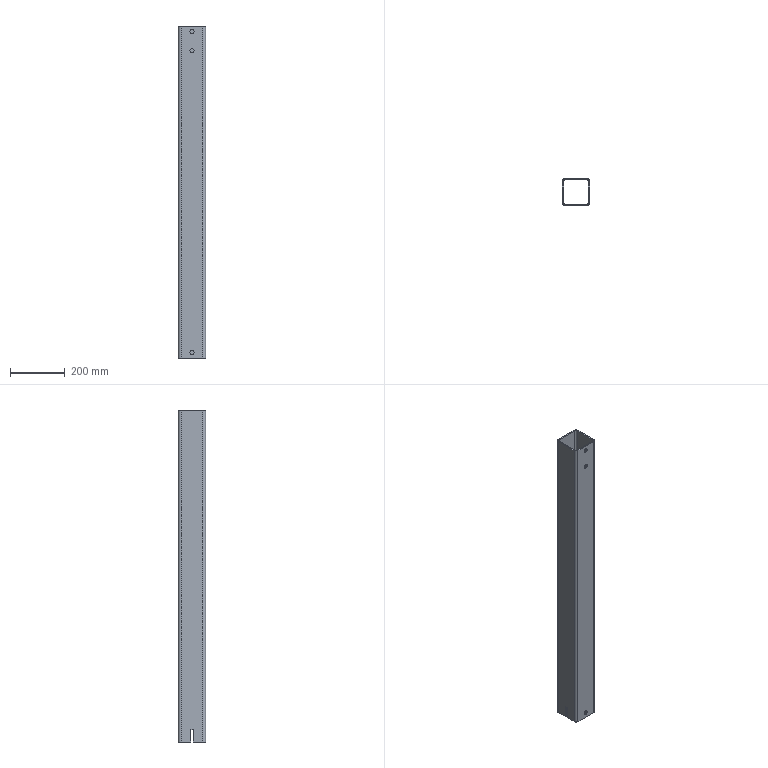Part | SolidWorks | features ICE 4, Attribute 1, Extrusion 1 | 1 solid | 39 faces | box 100 x 100 x 1211 mm | volume 1999990 mm3 | cylinder 22 | plane 17 | commonest cylinder face diameters 15 x14 11 x4 20 x4
STEP:
#1=CARTESIAN_POINT('',(-15.,45.5,1163.5));
#2=VERTEX_POINT('',#1);
#3=CARTESIAN_POINT('',(-15.,45.5,1178.5));
#4=VERTEX_POINT('',#3);
#5=CARTESIAN_POINT('',(-15.,45.5,1171.));
#6=DIRECTION('',(0.,1.,0.));
#7=DIRECTION('',(0.,0.,-1.));
#8=AXIS2_PLACEMENT_3D('',#5,#6,#7);
#9=CIRCLE('',#8,7.5);
#10=EDGE_CURVE('',#2,#4,#9,.T.);
#11=ORIENTED_EDGE('',*,*,#10,.F.);
#12=CARTESIAN_POINT('',(-15.,50.,1163.5));
#13=VERTEX_POINT('',#12);
#14=CARTESIAN_POINT('',(-15.,-50.001,1163.5));
#15=DIRECTION('',(0.,1.,0.));
#16=VECTOR('',#15,1000.);
#17=LINE('',#14,#16);
#18=EDGE_CURVE('',#2,#13,#17,.T.);
#19=ORIENTED_EDGE('',*,*,#18,.T.);
#20=CARTESIAN_POINT('',(-15.,50.,1178.5));
#21=VERTEX_POINT('',#20);
#22=CARTESIAN_POINT('',(-15.,50.,1171.));
#23=DIRECTION('',(0.,1.,0.));
#24=DIRECTION('',(0.,0.,1.));
#25=AXIS2_PLACEMENT_3D('',#22,#23,#24);
#26=CIRCLE('',#25,7.5);
#27=EDGE_CURVE('',#13,#21,#26,.T.);
#28=ORIENTED_EDGE('',*,*,#27,.T.);
#29=CARTESIAN_POINT('',(-15.,-50.001,1178.5));
#30=DIRECTION('',(0.,1.,0.));
#31=VECTOR('',#30,1000.);
#32=LINE('',#29,#31);
#33=EDGE_CURVE('',#4,#21,#32,.T.);
#34=ORIENTED_EDGE('',*,*,#33,.F.);
#35=EDGE_LOOP('',(#11,#19,#28,#34));
#36=FACE_OUTER_BOUND('',#35,.T.);
#37=CARTESIAN_POINT('',(-15.,-50.001,1171.));
#38=DIRECTION('',(0.,1.,0.));
#39=DIRECTION('',(0.,0.,1.));
#40=AXIS2_PLACEMENT_3D('',#37,#38,#39);
#41=CYLINDRICAL_SURFACE('',#40,7.5);
#42=ADVANCED_FACE('',(#36),#41,.F.);
#43=CARTESIAN_POINT('',(-15.,45.5,1113.5));
#44=VERTEX_POINT('',#43);
#45=CARTESIAN_POINT('',(-15.,45.5,1128.5));
#46=VERTEX_POINT('',#45);
#47=CARTESIAN_POINT('',(-15.,45.5,1121.));
#48=DIRECTION('',(0.,1.,0.));
#49=DIRECTION('',(0.,0.,-1.));
#50=AXIS2_PLACEMENT_3D('',#47,#48,#49);
#51=CIRCLE('',#50,7.5);
#52=EDGE_CURVE('',#44,#46,#51,.T.);
#53=ORIENTED_EDGE('',*,*,#52,.F.);
#54=CARTESIAN_POINT('',(-15.,50.,1113.5));
#55=VERTEX_POINT('',#54);
#56=CARTESIAN_POINT('',(-15.,-50.001,1113.5));
#57=DIRECTION('',(0.,1.,0.));
#58=VECTOR('',#57,1000.);
#59=LINE('',#56,#58);
#60=EDGE_CURVE('',#44,#55,#59,.T.);
#61=ORIENTED_EDGE('',*,*,#60,.T.);
#62=CARTESIAN_POINT('',(-15.,50.,1128.5));
#63=VERTEX_POINT('',#62);
#64=CARTESIAN_POINT('',(-15.,50.,1121.));
#65=DIRECTION('',(0.,1.,0.));
#66=DIRECTION('',(0.,0.,1.));
#67=AXIS2_PLACEMENT_3D('',#64,#65,#66);
#68=CIRCLE('',#67,7.5);
#69=EDGE_CURVE('',#55,#63,#68,.T.);
#70=ORIENTED_EDGE('',*,*,#69,.T.);
#71=CARTESIAN_POINT('',(-15.,-50.001,1128.5));
#72=DIRECTION('',(0.,1.,0.));
#73=VECTOR('',#72,1000.);
#74=LINE('',#71,#73);
#75=EDGE_CURVE('',#46,#63,#74,.T.);
#76=ORIENTED_EDGE('',*,*,#75,.F.);
#77=EDGE_LOOP('',(#53,#61,#70,#76));
#78=FACE_OUTER_BOUND('',#77,.T.);
#79=CARTESIAN_POINT('',(-15.,-50.001,1121.));
#80=DIRECTION('',(0.,1.,0.));
#81=DIRECTION('',(0.,0.,1.));
#82=AXIS2_PLACEMENT_3D('',#79,#80,#81);
#83=CYLINDRICAL_SURFACE('',#82,7.5);
#84=ADVANCED_FACE('',(#78),#83,.F.);
#85=CARTESIAN_POINT('',(0.,-45.5,1198.5));
#86=VERTEX_POINT('',#85);
#87=CARTESIAN_POINT('',(0.,-45.5,1183.5));
#88=VERTEX_POINT('',#87);
#89=CARTESIAN_POINT('',(0.,-45.5,1191.));
#90=DIRECTION('',(0.,-1.,0.));
#91=DIRECTION('',(0.,0.,1.));
#92=AXIS2_PLACEMENT_3D('',#89,#90,#91);
#93=CIRCLE('',#92,7.5);
#94=EDGE_CURVE('',#86,#88,#93,.T.);
#95=ORIENTED_EDGE('',*,*,#94,.F.);
#96=CARTESIAN_POINT('',(0.,-50.,1198.5));
#97=VERTEX_POINT('',#96);
#98=CARTESIAN_POINT('',(0.,50.001,1198.5));
#99=DIRECTION('',(0.,-1.,0.));
#100=VECTOR('',#99,1000.);
#101=LINE('',#98,#100);
#102=EDGE_CURVE('',#86,#97,#101,.T.);
#103=ORIENTED_EDGE('',*,*,#102,.T.);
#104=CARTESIAN_POINT('',(0.,-50.,1183.5));
#105=VERTEX_POINT('',#104);
#106=CARTESIAN_POINT('',(0.,-50.,1191.));
#107=DIRECTION('',(0.,-1.,0.));
#108=DIRECTION('',(0.,0.,-1.));
#109=AXIS2_PLACEMENT_3D('',#106,#107,#108);
#110=CIRCLE('',#109,7.5);
#111=EDGE_CURVE('',#97,#105,#110,.T.);
#112=ORIENTED_EDGE('',*,*,#111,.T.);
#113=CARTESIAN_POINT('',(0.,50.001,1183.5));
#114=DIRECTION('',(0.,-1.,0.));
#115=VECTOR('',#114,1000.);
#116=LINE('',#113,#115);
#117=EDGE_CURVE('',#88,#105,#116,.T.);
#118=ORIENTED_EDGE('',*,*,#117,.F.);
#119=EDGE_LOOP('',(#95,#103,#112,#118));
#120=FACE_OUTER_BOUND('',#119,.T.);
#121=CARTESIAN_POINT('',(0.,50.001,1191.));
#122=DIRECTION('',(0.,-1.,0.));
#123=DIRECTION('',(0.,0.,-1.));
#124=AXIS2_PLACEMENT_3D('',#121,#122,#123);
#125=CYLINDRICAL_SURFACE('',#124,7.5);
#126=ADVANCED_FACE('',(#120),#125,.F.);
#127=CARTESIAN_POINT('',(0.,-45.5,1128.5));
#128=VERTEX_POINT('',#127);
#129=CARTESIAN_POINT('',(0.,-45.5,1113.5));
#130=VERTEX_POINT('',#129);
#131=CARTESIAN_POINT('',(0.,-45.5,1121.));
#132=DIRECTION('',(0.,-1.,0.));
#133=DIRECTION('',(0.,0.,1.));
#134=AXIS2_PLACEMENT_3D('',#131,#132,#133);
#135=CIRCLE('',#134,7.5);
#136=EDGE_CURVE('',#128,#130,#135,.T.);
#137=ORIENTED_EDGE('',*,*,#136,.F.);
#138=CARTESIAN_POINT('',(0.,-50.,1128.5));
#139=VERTEX_POINT('',#138);
#140=CARTESIAN_POINT('',(0.,50.001,1128.5));
#141=DIRECTION('',(0.,-1.,0.));
#142=VECTOR('',#141,1000.);
#143=LINE('',#140,#142);
#144=EDGE_CURVE('',#128,#139,#143,.T.);
#145=ORIENTED_EDGE('',*,*,#144,.T.);
#146=CARTESIAN_POINT('',(0.,-50.,1113.5));
#147=VERTEX_POINT('',#146);
#148=CARTESIAN_POINT('',(0.,-50.,1121.));
#149=DIRECTION('',(0.,-1.,0.));
#150=DIRECTION('',(0.,0.,-1.));
#151=AXIS2_PLACEMENT_3D('',#148,#149,#150);
#152=CIRCLE('',#151,7.5);
#153=EDGE_CURVE('',#139,#147,#152,.T.);
#154=ORIENTED_EDGE('',*,*,#153,.T.);
#155=CARTESIAN_POINT('',(0.,50.001,1113.5));
#156=DIRECTION('',(0.,-1.,0.));
#157=VECTOR('',#156,1000.);
#158=LINE('',#155,#157);
#159=EDGE_CURVE('',#130,#147,#158,.T.);
#160=ORIENTED_EDGE('',*,*,#159,.F.);
#161=EDGE_LOOP('',(#137,#145,#154,#160));
#162=FACE_OUTER_BOUND('',#161,.T.);
#163=CARTESIAN_POINT('',(0.,50.001,1121.));
#164=DIRECTION('',(0.,-1.,0.));
#165=DIRECTION('',(0.,0.,-1.));
#166=AXIS2_PLACEMENT_3D('',#163,#164,#165);
#167=CYLINDRICAL_SURFACE('',#166,7.5);
#168=ADVANCED_FACE('',(#162),#167,.F.);
#169=CARTESIAN_POINT('',(0.,-45.5,27.5));
#170=VERTEX_POINT('',#169);
#171=CARTESIAN_POINT('',(0.,-45.5,12.5));
#172=VERTEX_POINT('',#171);
#173=CARTESIAN_POINT('',(0.,-45.5,20.));
#174=DIRECTION('',(0.,-1.,0.));
#175=DIRECTION('',(0.,0.,1.));
#176=AXIS2_PLACEMENT_3D('',#173,#174,#175);
#177=CIRCLE('',#176,7.5);
#178=EDGE_CURVE('',#170,#172,#177,.T.);
#179=ORIENTED_EDGE('',*,*,#178,.F.);
#180=CARTESIAN_POINT('',(0.,-50.,27.5));
#181=VERTEX_POINT('',#180);
#182=CARTESIAN_POINT('',(0.,50.001,27.5));
#183=DIRECTION('',(0.,-1.,0.));
#184=VECTOR('',#183,1000.);
#185=LINE('',#182,#184);
#186=EDGE_CURVE('',#170,#181,#185,.T.);
#187=ORIENTED_EDGE('',*,*,#186,.T.);
#188=CARTESIAN_POINT('',(0.,-50.,12.5));
#189=VERTEX_POINT('',#188);
#190=CARTESIAN_POINT('',(0.,-50.,20.));
#191=DIRECTION('',(0.,-1.,0.));
#192=DIRECTION('',(0.,0.,-1.));
#193=AXIS2_PLACEMENT_3D('',#190,#191,#192);
#194=CIRCLE('',#193,7.5);
#195=EDGE_CURVE('',#181,#189,#194,.T.);
#196=ORIENTED_EDGE('',*,*,#195,.T.);
#197=CARTESIAN_POINT('',(0.,50.001,12.5));
#198=DIRECTION('',(0.,-1.,0.));
#199=VECTOR('',#198,1000.);
#200=LINE('',#197,#199);
#201=EDGE_CURVE('',#172,#189,#200,.T.);
#202=ORIENTED_EDGE('',*,*,#201,.F.);
#203=EDGE_LOOP('',(#179,#187,#196,#202));
#204=FACE_OUTER_BOUND('',#203,.T.);
#205=CARTESIAN_POINT('',(0.,50.001,20.));
#206=DIRECTION('',(0.,-1.,0.));
#207=DIRECTION('',(0.,0.,-1.));
#208=AXIS2_PLACEMENT_3D('',#205,#206,#207);
#209=CYLINDRICAL_SURFACE('',#208,7.5);
#210=ADVANCED_FACE('',(#204),#209,.F.);
#211=CARTESIAN_POINT('',(45.5,-15.,1178.5));
#212=VERTEX_POINT('',#211);
#213=CARTESIAN_POINT('',(45.5,-15.,1163.5));
#214=VERTEX_POINT('',#213);
#215=CARTESIAN_POINT('',(45.5,-15.,1171.));
#216=DIRECTION('',(1.,0.,0.));
#217=DIRECTION('',(0.,0.,1.));
#218=AXIS2_PLACEMENT_3D('',#215,#216,#217);
#219=CIRCLE('',#218,7.5);
#220=EDGE_CURVE('',#212,#214,#219,.T.);
#221=ORIENTED_EDGE('',*,*,#220,.F.);
#222=CARTESIAN_POINT('',(50.,-15.,1178.5));
#223=VERTEX_POINT('',#222);
#224=CARTESIAN_POINT('',(-50.001,-15.,1178.5));
#225=DIRECTION('',(1.,0.,0.));
#226=VECTOR('',#225,1000.);
#227=LINE('',#224,#226);
#228=EDGE_CURVE('',#212,#223,#227,.T.);
#229=ORIENTED_EDGE('',*,*,#228,.T.);
#230=CARTESIAN_POINT('',(50.,-15.,1163.5));
#231=VERTEX_POINT('',#230);
#232=CARTESIAN_POINT('',(50.,-15.,1171.));
#233=DIRECTION('',(1.,0.,0.));
#234=DIRECTION('',(0.,0.,-1.));
#235=AXIS2_PLACEMENT_3D('',#232,#233,#234);
#236=CIRCLE('',#235,7.5);
#237=EDGE_CURVE('',#223,#231,#236,.T.);
#238=ORIENTED_EDGE('',*,*,#237,.T.);
#239=CARTESIAN_POINT('',(-50.001,-15.,1163.5));
#240=DIRECTION('',(1.,0.,0.));
#241=VECTOR('',#240,1000.);
#242=LINE('',#239,#241);
#243=EDGE_CURVE('',#214,#231,#242,.T.);
#244=ORIENTED_EDGE('',*,*,#243,.F.);
#245=EDGE_LOOP('',(#221,#229,#238,#244));
#246=FACE_OUTER_BOUND('',#245,.T.);
#247=CARTESIAN_POINT('',(-50.001,-15.,1171.));
#248=DIRECTION('',(1.,0.,0.));
#249=DIRECTION('',(0.,0.,-1.));
#250=AXIS2_PLACEMENT_3D('',#247,#248,#249);
#251=CYLINDRICAL_SURFACE('',#250,7.5);
#252=ADVANCED_FACE('',(#246),#251,.F.);
#253=CARTESIAN_POINT('',(45.5,-15.,1128.5));
#254=VERTEX_POINT('',#253);
#255=CARTESIAN_POINT('',(45.5,-15.,1113.5));
#256=VERTEX_POINT('',#255);
#257=CARTESIAN_POINT('',(45.5,-15.,1121.));
#258=DIRECTION('',(1.,0.,0.));
#259=DIRECTION('',(0.,0.,1.));
#260=AXIS2_PLACEMENT_3D('',#257,#258,#259);
#261=CIRCLE('',#260,7.5);
#262=EDGE_CURVE('',#254,#256,#261,.T.);
#263=ORIENTED_EDGE('',*,*,#262,.F.);
#264=CARTESIAN_POINT('',(50.,-15.,1128.5));
#265=VERTEX_POINT('',#264);
#266=CARTESIAN_POINT('',(-50.001,-15.,1128.5));
#267=DIRECTION('',(1.,0.,0.));
#268=VECTOR('',#267,1000.);
#269=LINE('',#266,#268);
#270=EDGE_CURVE('',#254,#265,#269,.T.);
#271=ORIENTED_EDGE('',*,*,#270,.T.);
#272=CARTESIAN_POINT('',(50.,-15.,1113.5));
#273=VERTEX_POINT('',#272);
#274=CARTESIAN_POINT('',(50.,-15.,1121.));
#275=DIRECTION('',(1.,0.,0.));
#276=DIRECTION('',(0.,0.,-1.));
#277=AXIS2_PLACEMENT_3D('',#274,#275,#276);
#278=CIRCLE('',#277,7.5);
#279=EDGE_CURVE('',#265,#273,#278,.T.);
#280=ORIENTED_EDGE('',*,*,#279,.T.);
#281=CARTESIAN_POINT('',(-50.001,-15.,1113.5));
#282=DIRECTION('',(1.,0.,0.));
#283=VECTOR('',#282,1000.);
#284=LINE('',#281,#283);
#285=EDGE_CURVE('',#256,#273,#284,.T.);
#286=ORIENTED_EDGE('',*,*,#285,.F.);
#287=EDGE_LOOP('',(#263,#271,#280,#286));
#288=FACE_OUTER_BOUND('',#287,.T.);
#289=CARTESIAN_POINT('',(-50.001,-15.,1121.));
#290=DIRECTION('',(1.,0.,0.));
#291=DIRECTION('',(0.,0.,-1.));
#292=AXIS2_PLACEMENT_3D('',#289,#290,#291);
#293=CYLINDRICAL_SURFACE('',#292,7.5);
#294=ADVANCED_FACE('',(#288),#293,.F.);
#295=CARTESIAN_POINT('',(-50.,-4.5,0.));
#296=VERTEX_POINT('',#295);
#297=CARTESIAN_POINT('',(-50.,-40.,0.));
#298=VERTEX_POINT('',#297);
#299=CARTESIAN_POINT('',(-50.,-40.,0.));
#300=DIRECTION('',(0.,-1.,0.));
#301=VECTOR('',#300,1000.);
#302=LINE('',#299,#301);
#303=EDGE_CURVE('',#296,#298,#302,.T.);
#304=ORIENTED_EDGE('',*,*,#303,.F.);
#305=CARTESIAN_POINT('',(-45.5,-4.5,0.));
#306=VERTEX_POINT('',#305);
#307=CARTESIAN_POINT('',(-50.,-4.5,0.));
#308=DIRECTION('',(1.,0.,0.));
#309=VECTOR('',#308,1000.);
#310=LINE('',#307,#309);
#311=EDGE_CURVE('',#296,#306,#310,.T.);
#312=ORIENTED_EDGE('',*,*,#311,.T.);
#313=CARTESIAN_POINT('',(-45.5,-40.,0.));
#314=VERTEX_POINT('',#313);
#315=CARTESIAN_POINT('',(-45.5,-40.,0.));
#316=DIRECTION('',(0.,-1.,0.));
#317=VECTOR('',#316,1000.);
#318=LINE('',#315,#317);
#319=EDGE_CURVE('',#306,#314,#318,.T.);
#320=ORIENTED_EDGE('',*,*,#319,.T.);
#321=CARTESIAN_POINT('',(-40.,-45.5,0.));
#322=VERTEX_POINT('',#321);
#323=CARTESIAN_POINT('',(-40.,-40.,0.));
#324=DIRECTION('',(0.,0.,1.));
#325=DIRECTION('',(1.,0.,0.));
#326=AXIS2_PLACEMENT_3D('',#323,#324,#325);
#327=CIRCLE('',#326,5.5);
#328=EDGE_CURVE('',#314,#322,#327,.T.);
#329=ORIENTED_EDGE('',*,*,#328,.T.);
#330=CARTESIAN_POINT('',(40.,-45.5,0.));
#331=VERTEX_POINT('',#330);
#332=CARTESIAN_POINT('',(-40.,-45.5,0.));
#333=DIRECTION('',(1.,0.,0.));
#334=VECTOR('',#333,1000.);
#335=LINE('',#332,#334);
#336=EDGE_CURVE('',#322,#331,#335,.T.);
#337=ORIENTED_EDGE('',*,*,#336,.T.);
#338=CARTESIAN_POINT('',(45.5,-40.,0.));
#339=VERTEX_POINT('',#338);
#340=CARTESIAN_POINT('',(40.,-40.,0.));
#341=DIRECTION('',(0.,0.,1.));
#342=DIRECTION('',(1.,0.,0.));
#343=AXIS2_PLACEMENT_3D('',#340,#341,#342);
#344=CIRCLE('',#343,5.5);
#345=EDGE_CURVE('',#331,#339,#344,.T.);
#346=ORIENTED_EDGE('',*,*,#345,.T.);
#347=CARTESIAN_POINT('',(45.5,-4.5,0.));
#348=VERTEX_POINT('',#347);
#349=CARTESIAN_POINT('',(45.5,40.,0.));
#350=DIRECTION('',(0.,1.,0.));
#351=VECTOR('',#350,1000.);
#352=LINE('',#349,#351);
#353=EDGE_CURVE('',#339,#348,#352,.T.);
#354=ORIENTED_EDGE('',*,*,#353,.T.);
#355=CARTESIAN_POINT('',(50.,-4.5,0.));
#356=VERTEX_POINT('',#355);
#357=CARTESIAN_POINT('',(-50.,-4.5,0.));
#358=DIRECTION('',(1.,0.,0.));
#359=VECTOR('',#358,1000.);
#360=LINE('',#357,#359);
#361=EDGE_CURVE('',#348,#356,#360,.T.);
#362=ORIENTED_EDGE('',*,*,#361,.T.);
#363=CARTESIAN_POINT('',(50.,-40.,0.));
#364=VERTEX_POINT('',#363);
#365=CARTESIAN_POINT('',(50.,40.,0.));
#366=DIRECTION('',(0.,1.,0.));
#367=VECTOR('',#366,1000.);
#368=LINE('',#365,#367);
#369=EDGE_CURVE('',#364,#356,#368,.T.);
#370=ORIENTED_EDGE('',*,*,#369,.F.);
#371=CARTESIAN_POINT('',(40.,-50.,0.));
#372=VERTEX_POINT('',#371);
#373=CARTESIAN_POINT('',(40.,-40.,0.));
#374=DIRECTION('',(0.,0.,1.));
#375=DIRECTION('',(1.,0.,0.));
#376=AXIS2_PLACEMENT_3D('',#373,#374,#375);
#377=CIRCLE('',#376,10.);
#378=EDGE_CURVE('',#372,#364,#377,.T.);
#379=ORIENTED_EDGE('',*,*,#378,.F.);
#380=CARTESIAN_POINT('',(-40.,-50.,0.));
#381=VERTEX_POINT('',#380);
#382=CARTESIAN_POINT('',(-40.,-50.,0.));
#383=DIRECTION('',(1.,0.,0.));
#384=VECTOR('',#383,1000.);
#385=LINE('',#382,#384);
#386=EDGE_CURVE('',#381,#372,#385,.T.);
#387=ORIENTED_EDGE('',*,*,#386,.F.);
#388=CARTESIAN_POINT('',(-40.,-40.,0.));
#389=DIRECTION('',(0.,0.,1.));
#390=DIRECTION('',(1.,0.,0.));
#391=AXIS2_PLACEMENT_3D('',#388,#389,#390);
#392=CIRCLE('',#391,10.);
#393=EDGE_CURVE('',#298,#381,#392,.T.);
#394=ORIENTED_EDGE('',*,*,#393,.F.);
#395=EDGE_LOOP('',(#304,#312,#320,#329,#337,#346,#354,#362,#370,#379,#387,#394));
#396=FACE_OUTER_BOUND('',#395,.T.);
#397=CARTESIAN_POINT('',(40.,40.,0.));
#398=DIRECTION('',(0.,0.,1.));
#399=DIRECTION('',(1.,0.,0.));
#400=AXIS2_PLACEMENT_3D('',#397,#398,#399);
#401=PLANE('',#400);
#402=ADVANCED_FACE('',(#396),#401,.F.);
#403=CARTESIAN_POINT('',(50.,40.,1211.));
#404=VERTEX_POINT('',#403);
#405=CARTESIAN_POINT('',(40.,50.,1211.));
#406=VERTEX_POINT('',#405);
#407=CARTESIAN_POINT('',(40.,40.,1211.));
#408=DIRECTION('',(0.,0.,1.));
#409=DIRECTION('',(1.,0.,0.));
#410=AXIS2_PLACEMENT_3D('',#407,#408,#409);
#411=CIRCLE('',#410,10.);
#412=EDGE_CURVE('',#404,#406,#411,.T.);
#413=ORIENTED_EDGE('',*,*,#412,.T.);
#414=CARTESIAN_POINT('',(-40.,50.,1211.));
#415=VERTEX_POINT('',#414);
#416=CARTESIAN_POINT('',(40.,50.,1211.));
#417=DIRECTION('',(-1.,0.,0.));
#418=VECTOR('',#417,1000.);
#419=LINE('',#416,#418);
#420=EDGE_CURVE('',#406,#415,#419,.T.);
#421=ORIENTED_EDGE('',*,*,#420,.T.);
#422=CARTESIAN_POINT('',(-50.,40.,1211.));
#423=VERTEX_POINT('',#422);
#424=CARTESIAN_POINT('',(-40.,40.,1211.));
#425=DIRECTION('',(0.,0.,1.));
#426=DIRECTION('',(1.,0.,0.));
#427=AXIS2_PLACEMENT_3D('',#424,#425,#426);
#428=CIRCLE('',#427,10.);
#429=EDGE_CURVE('',#415,#423,#428,.T.);
#430=ORIENTED_EDGE('',*,*,#429,.T.);
#431=CARTESIAN_POINT('',(-50.,-40.,1211.));
#432=VERTEX_POINT('',#431);
#433=CARTESIAN_POINT('',(-50.,-40.,1211.));
#434=DIRECTION('',(0.,-1.,0.));
#435=VECTOR('',#434,1000.);
#436=LINE('',#433,#435);
#437=EDGE_CURVE('',#423,#432,#436,.T.);
#438=ORIENTED_EDGE('',*,*,#437,.T.);
#439=CARTESIAN_POINT('',(-40.,-50.,1211.));
#440=VERTEX_POINT('',#439);
#441=CARTESIAN_POINT('',(-40.,-40.,1211.));
#442=DIRECTION('',(0.,0.,1.));
#443=DIRECTION('',(1.,0.,0.));
#444=AXIS2_PLACEMENT_3D('',#441,#442,#443);
#445=CIRCLE('',#444,10.);
#446=EDGE_CURVE('',#432,#440,#445,.T.);
#447=ORIENTED_EDGE('',*,*,#446,.T.);
#448=CARTESIAN_POINT('',(40.,-50.,1211.));
#449=VERTEX_POINT('',#448);
#450=CARTESIAN_POINT('',(-40.,-50.,1211.));
#451=DIRECTION('',(1.,0.,0.));
#452=VECTOR('',#451,1000.);
#453=LINE('',#450,#452);
#454=EDGE_CURVE('',#440,#449,#453,.T.);
#455=ORIENTED_EDGE('',*,*,#454,.T.);
#456=CARTESIAN_POINT('',(50.,-40.,1211.));
#457=VERTEX_POINT('',#456);
#458=CARTESIAN_POINT('',(40.,-40.,1211.));
#459=DIRECTION('',(0.,0.,1.));
#460=DIRECTION('',(1.,0.,0.));
#461=AXIS2_PLACEMENT_3D('',#458,#459,#460);
#462=CIRCLE('',#461,10.);
#463=EDGE_CURVE('',#449,#457,#462,.T.);
#464=ORIENTED_EDGE('',*,*,#463,.T.);
#465=CARTESIAN_POINT('',(50.,40.,1211.));
#466=DIRECTION('',(0.,1.,0.));
#467=VECTOR('',#466,1000.);
#468=LINE('',#465,#467);
#469=EDGE_CURVE('',#457,#404,#468,.T.);
#470=ORIENTED_EDGE('',*,*,#469,.T.);
#471=EDGE_LOOP('',(#413,#421,#430,#438,#447,#455,#464,#470));
#472=FACE_OUTER_BOUND('',#471,.T.);
#473=CARTESIAN_POINT('',(-45.5,40.,1211.));
#474=VERTEX_POINT('',#473);
#475=CARTESIAN_POINT('',(-45.5,-40.,1211.));
#476=VERTEX_POINT('',#475);
#477=CARTESIAN_POINT('',(-45.5,-40.,1211.));
#478=DIRECTION('',(0.,-1.,0.));
#479=VECTOR('',#478,1000.);
#480=LINE('',#477,#479);
#481=EDGE_CURVE('',#474,#476,#480,.T.);
#482=ORIENTED_EDGE('',*,*,#481,.F.);
#483=CARTESIAN_POINT('',(-40.,45.5,1211.));
#484=VERTEX_POINT('',#483);
#485=CARTESIAN_POINT('',(-40.,40.,1211.));
#486=DIRECTION('',(0.,0.,1.));
#487=DIRECTION('',(1.,0.,0.));
#488=AXIS2_PLACEMENT_3D('',#485,#486,#487);
#489=CIRCLE('',#488,5.5);
#490=EDGE_CURVE('',#484,#474,#489,.T.);
#491=ORIENTED_EDGE('',*,*,#490,.F.);
#492=CARTESIAN_POINT('',(40.,45.5,1211.));
#493=VERTEX_POINT('',#492);
#494=CARTESIAN_POINT('',(40.,45.5,1211.));
#495=DIRECTION('',(-1.,0.,0.));
#496=VECTOR('',#495,1000.);
#497=LINE('',#494,#496);
#498=EDGE_CURVE('',#493,#484,#497,.T.);
#499=ORIENTED_EDGE('',*,*,#498,.F.);
#500=CARTESIAN_POINT('',(45.5,40.,1211.));
#501=VERTEX_POINT('',#500);
#502=CARTESIAN_POINT('',(40.,40.,1211.));
#503=DIRECTION('',(0.,0.,1.));
#504=DIRECTION('',(1.,0.,0.));
#505=AXIS2_PLACEMENT_3D('',#502,#503,#504);
#506=CIRCLE('',#505,5.5);
#507=EDGE_CURVE('',#501,#493,#506,.T.);
#508=ORIENTED_EDGE('',*,*,#507,.F.);
#509=CARTESIAN_POINT('',(45.5,-40.,1211.));
#510=VERTEX_POINT('',#509);
#511=CARTESIAN_POINT('',(45.5,40.,1211.));
#512=DIRECTION('',(0.,1.,0.));
#513=VECTOR('',#512,1000.);
#514=LINE('',#511,#513);
#515=EDGE_CURVE('',#510,#501,#514,.T.);
#516=ORIENTED_EDGE('',*,*,#515,.F.);
#517=CARTESIAN_POINT('',(40.,-45.5,1211.));
#518=VERTEX_POINT('',#517);
#519=CARTESIAN_POINT('',(40.,-40.,1211.));
#520=DIRECTION('',(0.,0.,1.));
#521=DIRECTION('',(1.,0.,0.));
#522=AXIS2_PLACEMENT_3D('',#519,#520,#521);
#523=CIRCLE('',#522,5.5);
#524=EDGE_CURVE('',#518,#510,#523,.T.);
#525=ORIENTED_EDGE('',*,*,#524,.F.);
#526=CARTESIAN_POINT('',(-40.,-45.5,1211.));
#527=VERTEX_POINT('',#526);
#528=CARTESIAN_POINT('',(-40.,-45.5,1211.));
#529=DIRECTION('',(1.,0.,0.));
#530=VECTOR('',#529,1000.);
#531=LINE('',#528,#530);
#532=EDGE_CURVE('',#527,#518,#531,.T.);
#533=ORIENTED_EDGE('',*,*,#532,.F.);
#534=CARTESIAN_POINT('',(-40.,-40.,1211.));
#535=DIRECTION('',(0.,0.,1.));
#536=DIRECTION('',(1.,0.,0.));
#537=AXIS2_PLACEMENT_3D('',#534,#535,#536);
#538=CIRCLE('',#537,5.5);
#539=EDGE_CURVE('',#476,#527,#538,.T.);
#540=ORIENTED_EDGE('',*,*,#539,.F.);
#541=EDGE_LOOP('',(#482,#491,#499,#508,#516,#525,#533,#540));
#542=FACE_BOUND('',#541,.T.);
#543=CARTESIAN_POINT('',(40.,40.,1211.));
#544=DIRECTION('',(0.,0.,1.));
#545=DIRECTION('',(1.,0.,0.));
#546=AXIS2_PLACEMENT_3D('',#543,#544,#545);
#547=PLANE('',#546);
#548=ADVANCED_FACE('',(#472,#542),#547,.T.);
#549=CARTESIAN_POINT('',(50.,4.5,0.));
#550=VERTEX_POINT('',#549);
#551=CARTESIAN_POINT('',(50.,40.,0.));
#552=VERTEX_POINT('',#551);
#553=CARTESIAN_POINT('',(50.,40.,0.));
#554=DIRECTION('',(0.,1.,0.));
#555=VECTOR('',#554,1000.);
#556=LINE('',#553,#555);
#557=EDGE_CURVE('',#550,#552,#556,.T.);
#558=ORIENTED_EDGE('',*,*,#557,.F.);
#559=CARTESIAN_POINT('',(45.5,4.5,0.));
#560=VERTEX_POINT('',#559);
#561=CARTESIAN_POINT('',(-50.,4.5,0.));
#562=DIRECTION('',(1.,0.,0.));
#563=VECTOR('',#562,1000.);
#564=LINE('',#561,#563);
#565=EDGE_CURVE('',#560,#550,#564,.T.);
#566=ORIENTED_EDGE('',*,*,#565,.F.);
#567=CARTESIAN_POINT('',(45.5,40.,0.));
#568=VERTEX_POINT('',#567);
#569=CARTESIAN_POINT('',(45.5,40.,0.));
#570=DIRECTION('',(0.,1.,0.));
#571=VECTOR('',#570,1000.);
#572=LINE('',#569,#571);
#573=EDGE_CURVE('',#560,#568,#572,.T.);
#574=ORIENTED_EDGE('',*,*,#573,.T.);
#575=CARTESIAN_POINT('',(40.,45.5,0.));
#576=VERTEX_POINT('',#575);
#577=CARTESIAN_POINT('',(40.,40.,0.));
#578=DIRECTION('',(0.,0.,1.));
#579=DIRECTION('',(1.,0.,0.));
#580=AXIS2_PLACEMENT_3D('',#577,#578,#579);
#581=CIRCLE('',#580,5.5);
#582=EDGE_CURVE('',#568,#576,#581,.T.);
#583=ORIENTED_EDGE('',*,*,#582,.T.);
#584=CARTESIAN_POINT('',(-40.,45.5,0.));
#585=VERTEX_POINT('',#584);
#586=CARTESIAN_POINT('',(40.,45.5,0.));
#587=DIRECTION('',(-1.,0.,0.));
#588=VECTOR('',#587,1000.);
#589=LINE('',#586,#588);
#590=EDGE_CURVE('',#576,#585,#589,.T.);
#591=ORIENTED_EDGE('',*,*,#590,.T.);
#592=CARTESIAN_POINT('',(-45.5,40.,0.));
#593=VERTEX_POINT('',#592);
#594=CARTESIAN_POINT('',(-40.,40.,0.));
#595=DIRECTION('',(0.,0.,1.));
#596=DIRECTION('',(1.,0.,0.));
#597=AXIS2_PLACEMENT_3D('',#594,#595,#596);
#598=CIRCLE('',#597,5.5);
#599=EDGE_CURVE('',#585,#593,#598,.T.);
#600=ORIENTED_EDGE('',*,*,#599,.T.);
#601=CARTESIAN_POINT('',(-45.5,4.5,0.));
#602=VERTEX_POINT('',#601);
#603=CARTESIAN_POINT('',(-45.5,-40.,0.));
#604=DIRECTION('',(0.,-1.,0.));
#605=VECTOR('',#604,1000.);
#606=LINE('',#603,#605);
#607=EDGE_CURVE('',#593,#602,#606,.T.);
#608=ORIENTED_EDGE('',*,*,#607,.T.);
#609=CARTESIAN_POINT('',(-50.,4.5,0.));
#610=VERTEX_POINT('',#609);
#611=CARTESIAN_POINT('',(-50.,4.5,0.));
#612=DIRECTION('',(1.,0.,0.));
#613=VECTOR('',#612,1000.);
#614=LINE('',#611,#613);
#615=EDGE_CURVE('',#610,#602,#614,.T.);
#616=ORIENTED_EDGE('',*,*,#615,.F.);
#617=CARTESIAN_POINT('',(-50.,40.,0.));
#618=VERTEX_POINT('',#617);
#619=CARTESIAN_POINT('',(-50.,-40.,0.));
#620=DIRECTION('',(0.,-1.,0.));
#621=VECTOR('',#620,1000.);
#622=LINE('',#619,#621);
#623=EDGE_CURVE('',#618,#610,#622,.T.);
#624=ORIENTED_EDGE('',*,*,#623,.F.);
#625=CARTESIAN_POINT('',(-40.,50.,0.));
#626=VERTEX_POINT('',#625);
#627=CARTESIAN_POINT('',(-40.,40.,0.));
#628=DIRECTION('',(0.,0.,1.));
#629=DIRECTION('',(1.,0.,0.));
#630=AXIS2_PLACEMENT_3D('',#627,#628,#629);
#631=CIRCLE('',#630,10.);
#632=EDGE_CURVE('',#626,#618,#631,.T.);
#633=ORIENTED_EDGE('',*,*,#632,.F.);
#634=CARTESIAN_POINT('',(40.,50.,0.));
#635=VERTEX_POINT('',#634);
#636=CARTESIAN_POINT('',(40.,50.,0.));
#637=DIRECTION('',(-1.,0.,0.));
#638=VECTOR('',#637,1000.);
#639=LINE('',#636,#638);
#640=EDGE_CURVE('',#635,#626,#639,.T.);
#641=ORIENTED_EDGE('',*,*,#640,.F.);
#642=CARTESIAN_POINT('',(40.,40.,0.));
#643=DIRECTION('',(0.,0.,1.));
#644=DIRECTION('',(1.,0.,0.));
#645=AXIS2_PLACEMENT_3D('',#642,#643,#644);
#646=CIRCLE('',#645,10.);
#647=EDGE_CURVE('',#552,#635,#646,.T.);
#648=ORIENTED_EDGE('',*,*,#647,.F.);
#649=EDGE_LOOP('',(#558,#566,#574,#583,#591,#600,#608,#616,#624,#633,#641,#648));
#650=FACE_OUTER_BOUND('',#649,.T.);
#651=CARTESIAN_POINT('',(40.,40.,0.));
#652=DIRECTION('',(0.,0.,1.));
#653=DIRECTION('',(1.,0.,0.));
#654=AXIS2_PLACEMENT_3D('',#651,#652,#653);
#655=PLANE('',#654);
#656=ADVANCED_FACE('',(#650),#655,.F.);
#657=ORIENTED_EDGE('',*,*,#647,.T.);
#658=CARTESIAN_POINT('',(40.,50.,1211.));
#659=DIRECTION('',(0.,0.,-1.));
#660=VECTOR('',#659,1000.);
#661=LINE('',#658,#660);
#662=EDGE_CURVE('',#406,#635,#661,.T.);
#663=ORIENTED_EDGE('',*,*,#662,.F.);
#664=ORIENTED_EDGE('',*,*,#412,.F.);
#665=CARTESIAN_POINT('',(50.,40.,1211.));
#666=DIRECTION('',(0.,0.,-1.));
#667=VECTOR('',#666,1000.);
#668=LINE('',#665,#667);
#669=EDGE_CURVE('',#404,#552,#668,.T.);
#670=ORIENTED_EDGE('',*,*,#669,.T.);
#671=EDGE_LOOP('',(#657,#663,#664,#670));
#672=FACE_OUTER_BOUND('',#671,.T.);
#673=CARTESIAN_POINT('',(40.,40.,1211.));
#674=DIRECTION('',(0.,0.,-1.));
#675=DIRECTION('',(-1.,0.,0.));
#676=AXIS2_PLACEMENT_3D('',#673,#674,#675);
#677=CYLINDRICAL_SURFACE('',#676,10.);
#678=ADVANCED_FACE('',(#672),#677,.T.);
#679=CARTESIAN_POINT('',(-15.,50.,1171.));
#680=DIRECTION('',(0.,1.,0.));
#681=DIRECTION('',(0.,0.,1.));
#682=AXIS2_PLACEMENT_3D('',#679,#680,#681);
#683=CIRCLE('',#682,7.5);
#684=EDGE_CURVE('',#21,#13,#683,.T.);
#685=ORIENTED_EDGE('',*,*,#684,.F.);
#686=ORIENTED_EDGE('',*,*,#27,.F.);
#687=EDGE_LOOP('',(#685,#686));
#688=FACE_BOUND('',#687,.T.);
#689=CARTESIAN_POINT('',(-15.,50.,1121.));
#690=DIRECTION('',(0.,1.,0.));
#691=DIRECTION('',(0.,0.,1.));
#692=AXIS2_PLACEMENT_3D('',#689,#690,#691);
#693=CIRCLE('',#692,7.5);
#694=EDGE_CURVE('',#63,#55,#693,.T.);
#695=ORIENTED_EDGE('',*,*,#694,.F.);
#696=ORIENTED_EDGE('',*,*,#69,.F.);
#697=EDGE_LOOP('',(#695,#696));
#698=FACE_BOUND('',#697,.T.);
#699=ORIENTED_EDGE('',*,*,#640,.T.);
#700=CARTESIAN_POINT('',(-40.,50.,1211.));
#701=DIRECTION('',(0.,0.,-1.));
#702=VECTOR('',#701,1000.);
#703=LINE('',#700,#702);
#704=EDGE_CURVE('',#415,#626,#703,.T.);
#705=ORIENTED_EDGE('',*,*,#704,.F.);
#706=ORIENTED_EDGE('',*,*,#420,.F.);
#707=ORIENTED_EDGE('',*,*,#662,.T.);
#708=EDGE_LOOP('',(#699,#705,#706,#707));
#709=FACE_OUTER_BOUND('',#708,.T.);
#710=CARTESIAN_POINT('',(40.,50.,1211.));
#711=DIRECTION('',(0.,-1.,0.));
#712=DIRECTION('',(0.,0.,-1.));
#713=AXIS2_PLACEMENT_3D('',#710,#711,#712);
#714=PLANE('',#713);
#715=ADVANCED_FACE('',(#688,#698,#709),#714,.F.);
#716=ORIENTED_EDGE('',*,*,#632,.T.);
#717=CARTESIAN_POINT('',(-50.,40.,1211.));
#718=DIRECTION('',(0.,0.,-1.));
#719=VECTOR('',#718,1000.);
#720=LINE('',#717,#719);
#721=EDGE_CURVE('',#423,#618,#720,.T.);
#722=ORIENTED_EDGE('',*,*,#721,.F.);
#723=ORIENTED_EDGE('',*,*,#429,.F.);
#724=ORIENTED_EDGE('',*,*,#704,.T.);
#725=EDGE_LOOP('',(#716,#722,#723,#724));
#726=FACE_OUTER_BOUND('',#725,.T.);
#727=CARTESIAN_POINT('',(-40.,40.,1211.));
#728=DIRECTION('',(0.,0.,-1.));
#729=DIRECTION('',(-1.,0.,0.));
#730=AXIS2_PLACEMENT_3D('',#727,#728,#729);
#731=CYLINDRICAL_SURFACE('',#730,10.);
#732=ADVANCED_FACE('',(#726),#731,.T.);
#733=CARTESIAN_POINT('',(-50.,4.5,45.));
#734=VERTEX_POINT('',#733);
#735=CARTESIAN_POINT('',(-50.,-4.5,45.));
#736=VERTEX_POINT('',#735);
#737=CARTESIAN_POINT('',(-50.,-4.5,45.));
#738=DIRECTION('',(0.,-1.,0.));
#739=VECTOR('',#738,1000.);
#740=LINE('',#737,#739);
#741=EDGE_CURVE('',#734,#736,#740,.T.);
#742=ORIENTED_EDGE('',*,*,#741,.T.);
#743=CARTESIAN_POINT('',(-50.,-4.5,0.));
#744=DIRECTION('',(0.,0.,-1.));
#745=VECTOR('',#744,1000.);
#746=LINE('',#743,#745);
#747=EDGE_CURVE('',#736,#296,#746,.T.);
#748=ORIENTED_EDGE('',*,*,#747,.T.);
#749=ORIENTED_EDGE('',*,*,#303,.T.);
#750=CARTESIAN_POINT('',(-50.,-40.,1211.));
#751=DIRECTION('',(0.,0.,-1.));
#752=VECTOR('',#751,1000.);
#753=LINE('',#750,#752);
#754=EDGE_CURVE('',#432,#298,#753,.T.);
#755=ORIENTED_EDGE('',*,*,#754,.F.);
#756=ORIENTED_EDGE('',*,*,#437,.F.);
#757=ORIENTED_EDGE('',*,*,#721,.T.);
#758=ORIENTED_EDGE('',*,*,#623,.T.);
#759=CARTESIAN_POINT('',(-50.,4.5,0.));
#760=DIRECTION('',(0.,0.,1.));
#761=VECTOR('',#760,1000.);
#762=LINE('',#759,#761);
#763=EDGE_CURVE('',#610,#734,#762,.T.);
#764=ORIENTED_EDGE('',*,*,#763,.T.);
#765=EDGE_LOOP('',(#742,#748,#749,#755,#756,#757,#758,#764));
#766=FACE_OUTER_BOUND('',#765,.T.);
#767=CARTESIAN_POINT('',(-50.,-40.,1211.));
#768=DIRECTION('',(1.,0.,0.));
#769=DIRECTION('',(0.,0.,-1.));
#770=AXIS2_PLACEMENT_3D('',#767,#768,#769);
#771=PLANE('',#770);
#772=ADVANCED_FACE('',(#766),#771,.F.);
#773=ORIENTED_EDGE('',*,*,#393,.T.);
#774=CARTESIAN_POINT('',(-40.,-50.,1211.));
#775=DIRECTION('',(0.,0.,-1.));
#776=VECTOR('',#775,1000.);
#777=LINE('',#774,#776);
#778=EDGE_CURVE('',#440,#381,#777,.T.);
#779=ORIENTED_EDGE('',*,*,#778,.F.);
#780=ORIENTED_EDGE('',*,*,#446,.F.);
#781=ORIENTED_EDGE('',*,*,#754,.T.);
#782=EDGE_LOOP('',(#773,#779,#780,#781));
#783=FACE_OUTER_BOUND('',#782,.T.);
#784=CARTESIAN_POINT('',(-40.,-40.,1211.));
#785=DIRECTION('',(0.,0.,-1.));
#786=DIRECTION('',(-1.,0.,0.));
#787=AXIS2_PLACEMENT_3D('',#784,#785,#786);
#788=CYLINDRICAL_SURFACE('',#787,10.);
#789=ADVANCED_FACE('',(#783),#788,.T.);
#790=CARTESIAN_POINT('',(0.,-50.,1191.));
#791=DIRECTION('',(0.,-1.,0.));
#792=DIRECTION('',(0.,0.,-1.));
#793=AXIS2_PLACEMENT_3D('',#790,#791,#792);
#794=CIRCLE('',#793,7.5);
#795=EDGE_CURVE('',#105,#97,#794,.T.);
#796=ORIENTED_EDGE('',*,*,#795,.F.);
#797=ORIENTED_EDGE('',*,*,#111,.F.);
#798=EDGE_LOOP('',(#796,#797));
#799=FACE_BOUND('',#798,.T.);
#800=CARTESIAN_POINT('',(0.,-50.,1121.));
#801=DIRECTION('',(0.,-1.,0.));
#802=DIRECTION('',(0.,0.,-1.));
#803=AXIS2_PLACEMENT_3D('',#800,#801,#802);
#804=CIRCLE('',#803,7.5);
#805=EDGE_CURVE('',#147,#139,#804,.T.);
#806=ORIENTED_EDGE('',*,*,#805,.F.);
#807=ORIENTED_EDGE('',*,*,#153,.F.);
#808=EDGE_LOOP('',(#806,#807));
#809=FACE_BOUND('',#808,.T.);
#810=CARTESIAN_POINT('',(0.,-50.,20.));
#811=DIRECTION('',(0.,-1.,0.));
#812=DIRECTION('',(0.,0.,-1.));
#813=AXIS2_PLACEMENT_3D('',#810,#811,#812);
#814=CIRCLE('',#813,7.5);
#815=EDGE_CURVE('',#189,#181,#814,.T.);
#816=ORIENTED_EDGE('',*,*,#815,.F.);
#817=ORIENTED_EDGE('',*,*,#195,.F.);
#818=EDGE_LOOP('',(#816,#817));
#819=FACE_BOUND('',#818,.T.);
#820=ORIENTED_EDGE('',*,*,#386,.T.);
#821=CARTESIAN_POINT('',(40.,-50.,1211.));
#822=DIRECTION('',(0.,0.,-1.));
#823=VECTOR('',#822,1000.);
#824=LINE('',#821,#823);
#825=EDGE_CURVE('',#449,#372,#824,.T.);
#826=ORIENTED_EDGE('',*,*,#825,.F.);
#827=ORIENTED_EDGE('',*,*,#454,.F.);
#828=ORIENTED_EDGE('',*,*,#778,.T.);
#829=EDGE_LOOP('',(#820,#826,#827,#828));
#830=FACE_OUTER_BOUND('',#829,.T.);
#831=CARTESIAN_POINT('',(-40.,-50.,1211.));
#832=DIRECTION('',(0.,1.,0.));
#833=DIRECTION('',(0.,0.,1.));
#834=AXIS2_PLACEMENT_3D('',#831,#832,#833);
#835=PLANE('',#834);
#836=ADVANCED_FACE('',(#799,#809,#819,#830),#835,.F.);
#837=ORIENTED_EDGE('',*,*,#378,.T.);
#838=CARTESIAN_POINT('',(50.,-40.,1211.));
#839=DIRECTION('',(0.,0.,-1.));
#840=VECTOR('',#839,1000.);
#841=LINE('',#838,#840);
#842=EDGE_CURVE('',#457,#364,#841,.T.);
#843=ORIENTED_EDGE('',*,*,#842,.F.);
#844=ORIENTED_EDGE('',*,*,#463,.F.);
#845=ORIENTED_EDGE('',*,*,#825,.T.);
#846=EDGE_LOOP('',(#837,#843,#844,#845));
#847=FACE_OUTER_BOUND('',#846,.T.);
#848=CARTESIAN_POINT('',(40.,-40.,1211.));
#849=DIRECTION('',(0.,0.,-1.));
#850=DIRECTION('',(-1.,0.,0.));
#851=AXIS2_PLACEMENT_3D('',#848,#849,#850);
#852=CYLINDRICAL_SURFACE('',#851,10.);
#853=ADVANCED_FACE('',(#847),#852,.T.);
#854=CARTESIAN_POINT('',(50.,-15.,1171.));
#855=DIRECTION('',(1.,0.,0.));
#856=DIRECTION('',(0.,0.,-1.));
#857=AXIS2_PLACEMENT_3D('',#854,#855,#856);
#858=CIRCLE('',#857,7.5);
#859=EDGE_CURVE('',#231,#223,#858,.T.);
#860=ORIENTED_EDGE('',*,*,#859,.F.);
#861=ORIENTED_EDGE('',*,*,#237,.F.);
#862=EDGE_LOOP('',(#860,#861));
#863=FACE_BOUND('',#862,.T.);
#864=CARTESIAN_POINT('',(50.,-15.,1121.));
#865=DIRECTION('',(1.,0.,0.));
#866=DIRECTION('',(0.,0.,-1.));
#867=AXIS2_PLACEMENT_3D('',#864,#865,#866);
#868=CIRCLE('',#867,7.5);
#869=EDGE_CURVE('',#273,#265,#868,.T.);
#870=ORIENTED_EDGE('',*,*,#869,.F.);
#871=ORIENTED_EDGE('',*,*,#279,.F.);
#872=EDGE_LOOP('',(#870,#871));
#873=FACE_BOUND('',#872,.T.);
#874=ORIENTED_EDGE('',*,*,#369,.T.);
#875=CARTESIAN_POINT('',(50.,-4.5,45.));
#876=VERTEX_POINT('',#875);
#877=CARTESIAN_POINT('',(50.,-4.5,0.));
#878=DIRECTION('',(0.,0.,-1.));
#879=VECTOR('',#878,1000.);
#880=LINE('',#877,#879);
#881=EDGE_CURVE('',#876,#356,#880,.T.);
#882=ORIENTED_EDGE('',*,*,#881,.F.);
#883=CARTESIAN_POINT('',(50.,4.5,45.));
#884=VERTEX_POINT('',#883);
#885=CARTESIAN_POINT('',(50.,-4.5,45.));
#886=DIRECTION('',(0.,-1.,0.));
#887=VECTOR('',#886,1000.);
#888=LINE('',#885,#887);
#889=EDGE_CURVE('',#884,#876,#888,.T.);
#890=ORIENTED_EDGE('',*,*,#889,.F.);
#891=CARTESIAN_POINT('',(50.,4.5,0.));
#892=DIRECTION('',(0.,0.,1.));
#893=VECTOR('',#892,1000.);
#894=LINE('',#891,#893);
#895=EDGE_CURVE('',#550,#884,#894,.T.);
#896=ORIENTED_EDGE('',*,*,#895,.F.);
#897=ORIENTED_EDGE('',*,*,#557,.T.);
#898=ORIENTED_EDGE('',*,*,#669,.F.);
#899=ORIENTED_EDGE('',*,*,#469,.F.);
#900=ORIENTED_EDGE('',*,*,#842,.T.);
#901=EDGE_LOOP('',(#874,#882,#890,#896,#897,#898,#899,#900));
#902=FACE_OUTER_BOUND('',#901,.T.);
#903=CARTESIAN_POINT('',(50.,40.,1211.));
#904=DIRECTION('',(-1.,0.,0.));
#905=DIRECTION('',(0.,0.,1.));
#906=AXIS2_PLACEMENT_3D('',#903,#904,#905);
#907=PLANE('',#906);
#908=ADVANCED_FACE('',(#863,#873,#902),#907,.F.);
#909=ORIENTED_EDGE('',*,*,#599,.F.);
#910=CARTESIAN_POINT('',(-40.,45.5,1211.));
#911=DIRECTION('',(0.,0.,-1.));
#912=VECTOR('',#911,1000.);
#913=LINE('',#910,#912);
#914=EDGE_CURVE('',#484,#585,#913,.T.);
#915=ORIENTED_EDGE('',*,*,#914,.F.);
#916=ORIENTED_EDGE('',*,*,#490,.T.);
#917=CARTESIAN_POINT('',(-45.5,40.,1211.));
#918=DIRECTION('',(0.,0.,-1.));
#919=VECTOR('',#918,1000.);
#920=LINE('',#917,#919);
#921=EDGE_CURVE('',#474,#593,#920,.T.);
#922=ORIENTED_EDGE('',*,*,#921,.T.);
#923=EDGE_LOOP('',(#909,#915,#916,#922));
#924=FACE_OUTER_BOUND('',#923,.T.);
#925=CARTESIAN_POINT('',(-40.,40.,1211.));
#926=DIRECTION('',(0.,0.,-1.));
#927=DIRECTION('',(-1.,0.,0.));
#928=AXIS2_PLACEMENT_3D('',#925,#926,#927);
#929=CYLINDRICAL_SURFACE('',#928,5.5);
#930=ADVANCED_FACE('',(#924),#929,.F.);
#931=CARTESIAN_POINT('',(-45.5,-4.5,45.));
#932=VERTEX_POINT('',#931);
#933=CARTESIAN_POINT('',(-45.5,-4.5,1211.));
#934=DIRECTION('',(0.,0.,-1.));
#935=VECTOR('',#934,1000.);
#936=LINE('',#933,#935);
#937=EDGE_CURVE('',#932,#306,#936,.T.);
#938=ORIENTED_EDGE('',*,*,#937,.F.);
#939=CARTESIAN_POINT('',(-45.5,4.5,45.));
#940=VERTEX_POINT('',#939);
#941=CARTESIAN_POINT('',(-45.5,-40.,45.));
#942=DIRECTION('',(0.,-1.,0.));
#943=VECTOR('',#942,1000.);
#944=LINE('',#941,#943);
#945=EDGE_CURVE('',#940,#932,#944,.T.);
#946=ORIENTED_EDGE('',*,*,#945,.F.);
#947=CARTESIAN_POINT('',(-45.5,4.5,1211.));
#948=DIRECTION('',(0.,0.,1.));
#949=VECTOR('',#948,1000.);
#950=LINE('',#947,#949);
#951=EDGE_CURVE('',#602,#940,#950,.T.);
#952=ORIENTED_EDGE('',*,*,#951,.F.);
#953=ORIENTED_EDGE('',*,*,#607,.F.);
#954=ORIENTED_EDGE('',*,*,#921,.F.);
#955=ORIENTED_EDGE('',*,*,#481,.T.);
#956=CARTESIAN_POINT('',(-45.5,-40.,1211.));
#957=DIRECTION('',(0.,0.,-1.));
#958=VECTOR('',#957,1000.);
#959=LINE('',#956,#958);
#960=EDGE_CURVE('',#476,#314,#959,.T.);
#961=ORIENTED_EDGE('',*,*,#960,.T.);
#962=ORIENTED_EDGE('',*,*,#319,.F.);
#963=EDGE_LOOP('',(#938,#946,#952,#953,#954,#955,#961,#962));
#964=FACE_OUTER_BOUND('',#963,.T.);
#965=CARTESIAN_POINT('',(-45.5,-40.,1211.));
#966=DIRECTION('',(1.,0.,0.));
#967=DIRECTION('',(0.,0.,-1.));
#968=AXIS2_PLACEMENT_3D('',#965,#966,#967);
#969=PLANE('',#968);
#970=ADVANCED_FACE('',(#964),#969,.T.);
#971=ORIENTED_EDGE('',*,*,#328,.F.);
#972=ORIENTED_EDGE('',*,*,#960,.F.);
#973=ORIENTED_EDGE('',*,*,#539,.T.);
#974=CARTESIAN_POINT('',(-40.,-45.5,1211.));
#975=DIRECTION('',(0.,0.,-1.));
#976=VECTOR('',#975,1000.);
#977=LINE('',#974,#976);
#978=EDGE_CURVE('',#527,#322,#977,.T.);
#979=ORIENTED_EDGE('',*,*,#978,.T.);
#980=EDGE_LOOP('',(#971,#972,#973,#979));
#981=FACE_OUTER_BOUND('',#980,.T.);
#982=CARTESIAN_POINT('',(-40.,-40.,1211.));
#983=DIRECTION('',(0.,0.,-1.));
#984=DIRECTION('',(-1.,0.,0.));
#985=AXIS2_PLACEMENT_3D('',#982,#983,#984);
#986=CYLINDRICAL_SURFACE('',#985,5.5);
#987=ADVANCED_FACE('',(#981),#986,.F.);
#988=CARTESIAN_POINT('',(0.,-45.5,1191.));
#989=DIRECTION('',(0.,-1.,0.));
#990=DIRECTION('',(0.,0.,1.));
#991=AXIS2_PLACEMENT_3D('',#988,#989,#990);
#992=CIRCLE('',#991,7.5);
#993=EDGE_CURVE('',#88,#86,#992,.T.);
#994=ORIENTED_EDGE('',*,*,#993,.T.);
#995=ORIENTED_EDGE('',*,*,#94,.T.);
#996=EDGE_LOOP('',(#994,#995));
#997=FACE_BOUND('',#996,.T.);
#998=CARTESIAN_POINT('',(0.,-45.5,1121.));
#999=DIRECTION('',(0.,-1.,0.));
#1000=DIRECTION('',(0.,0.,1.));
#1001=AXIS2_PLACEMENT_3D('',#998,#999,#1000);
#1002=CIRCLE('',#1001,7.5);
#1003=EDGE_CURVE('',#130,#128,#1002,.T.);
#1004=ORIENTED_EDGE('',*,*,#1003,.T.);
#1005=ORIENTED_EDGE('',*,*,#136,.T.);
#1006=EDGE_LOOP('',(#1004,#1005));
#1007=FACE_BOUND('',#1006,.T.);
#1008=CARTESIAN_POINT('',(0.,-45.5,20.));
#1009=DIRECTION('',(0.,-1.,0.));
#1010=DIRECTION('',(0.,0.,1.));
#1011=AXIS2_PLACEMENT_3D('',#1008,#1009,#1010);
#1012=CIRCLE('',#1011,7.5);
#1013=EDGE_CURVE('',#172,#170,#1012,.T.);
#1014=ORIENTED_EDGE('',*,*,#1013,.T.);
#1015=ORIENTED_EDGE('',*,*,#178,.T.);
#1016=EDGE_LOOP('',(#1014,#1015));
#1017=FACE_BOUND('',#1016,.T.);
#1018=ORIENTED_EDGE('',*,*,#336,.F.);
#1019=ORIENTED_EDGE('',*,*,#978,.F.);
#1020=ORIENTED_EDGE('',*,*,#532,.T.);
#1021=CARTESIAN_POINT('',(40.,-45.5,1211.));
#1022=DIRECTION('',(0.,0.,-1.));
#1023=VECTOR('',#1022,1000.);
#1024=LINE('',#1021,#1023);
#1025=EDGE_CURVE('',#518,#331,#1024,.T.);
#1026=ORIENTED_EDGE('',*,*,#1025,.T.);
#1027=EDGE_LOOP('',(#1018,#1019,#1020,#1026));
#1028=FACE_OUTER_BOUND('',#1027,.T.);
#1029=CARTESIAN_POINT('',(-40.,-45.5,1211.));
#1030=DIRECTION('',(0.,1.,0.));
#1031=DIRECTION('',(0.,0.,1.));
#1032=AXIS2_PLACEMENT_3D('',#1029,#1030,#1031);
#1033=PLANE('',#1032);
#1034=ADVANCED_FACE('',(#997,#1007,#1017,#1028),#1033,.T.);
#1035=ORIENTED_EDGE('',*,*,#345,.F.);
#1036=ORIENTED_EDGE('',*,*,#1025,.F.);
#1037=ORIENTED_EDGE('',*,*,#524,.T.);
#1038=CARTESIAN_POINT('',(45.5,-40.,1211.));
#1039=DIRECTION('',(0.,0.,-1.));
#1040=VECTOR('',#1039,1000.);
#1041=LINE('',#1038,#1040);
#1042=EDGE_CURVE('',#510,#339,#1041,.T.);
#1043=ORIENTED_EDGE('',*,*,#1042,.T.);
#1044=EDGE_LOOP('',(#1035,#1036,#1037,#1043));
#1045=FACE_OUTER_BOUND('',#1044,.T.);
#1046=CARTESIAN_POINT('',(40.,-40.,1211.));
#1047=DIRECTION('',(0.,0.,-1.));
#1048=DIRECTION('',(-1.,0.,0.));
#1049=AXIS2_PLACEMENT_3D('',#1046,#1047,#1048);
#1050=CYLINDRICAL_SURFACE('',#1049,5.5);
#1051=ADVANCED_FACE('',(#1045),#1050,.F.);
#1052=CARTESIAN_POINT('',(45.5,-4.5,45.));
#1053=VERTEX_POINT('',#1052);
#1054=CARTESIAN_POINT('',(45.5,-4.5,1211.));
#1055=DIRECTION('',(0.,0.,1.));
#1056=VECTOR('',#1055,1000.);
#1057=LINE('',#1054,#1056);
#1058=EDGE_CURVE('',#348,#1053,#1057,.T.);
#1059=ORIENTED_EDGE('',*,*,#1058,.F.);
#1060=ORIENTED_EDGE('',*,*,#353,.F.);
#1061=ORIENTED_EDGE('',*,*,#1042,.F.);
#1062=ORIENTED_EDGE('',*,*,#515,.T.);
#1063=CARTESIAN_POINT('',(45.5,40.,1211.));
#1064=DIRECTION('',(0.,0.,-1.));
#1065=VECTOR('',#1064,1000.);
#1066=LINE('',#1063,#1065);
#1067=EDGE_CURVE('',#501,#568,#1066,.T.);
#1068=ORIENTED_EDGE('',*,*,#1067,.T.);
#1069=ORIENTED_EDGE('',*,*,#573,.F.);
#1070=CARTESIAN_POINT('',(45.5,4.5,45.));
#1071=VERTEX_POINT('',#1070);
#1072=CARTESIAN_POINT('',(45.5,4.5,1211.));
#1073=DIRECTION('',(0.,0.,-1.));
#1074=VECTOR('',#1073,1000.);
#1075=LINE('',#1072,#1074);
#1076=EDGE_CURVE('',#1071,#560,#1075,.T.);
#1077=ORIENTED_EDGE('',*,*,#1076,.F.);
#1078=CARTESIAN_POINT('',(45.5,40.,45.));
#1079=DIRECTION('',(0.,1.,0.));
#1080=VECTOR('',#1079,1000.);
#1081=LINE('',#1078,#1080);
#1082=EDGE_CURVE('',#1053,#1071,#1081,.T.);
#1083=ORIENTED_EDGE('',*,*,#1082,.F.);
#1084=EDGE_LOOP('',(#1059,#1060,#1061,#1062,#1068,#1069,#1077,#1083));
#1085=FACE_OUTER_BOUND('',#1084,.T.);
#1086=CARTESIAN_POINT('',(45.5,-15.,1171.));
#1087=DIRECTION('',(1.,0.,0.));
#1088=DIRECTION('',(0.,0.,1.));
#1089=AXIS2_PLACEMENT_3D('',#1086,#1087,#1088);
#1090=CIRCLE('',#1089,7.5);
#1091=EDGE_CURVE('',#214,#212,#1090,.T.);
#1092=ORIENTED_EDGE('',*,*,#1091,.T.);
#1093=ORIENTED_EDGE('',*,*,#220,.T.);
#1094=EDGE_LOOP('',(#1092,#1093));
#1095=FACE_BOUND('',#1094,.T.);
#1096=CARTESIAN_POINT('',(45.5,-15.,1121.));
#1097=DIRECTION('',(1.,0.,0.));
#1098=DIRECTION('',(0.,0.,1.));
#1099=AXIS2_PLACEMENT_3D('',#1096,#1097,#1098);
#1100=CIRCLE('',#1099,7.5);
#1101=EDGE_CURVE('',#256,#254,#1100,.T.);
#1102=ORIENTED_EDGE('',*,*,#1101,.T.);
#1103=ORIENTED_EDGE('',*,*,#262,.T.);
#1104=EDGE_LOOP('',(#1102,#1103));
#1105=FACE_BOUND('',#1104,.T.);
#1106=CARTESIAN_POINT('',(45.5,40.,1211.));
#1107=DIRECTION('',(-1.,0.,0.));
#1108=DIRECTION('',(0.,0.,1.));
#1109=AXIS2_PLACEMENT_3D('',#1106,#1107,#1108);
#1110=PLANE('',#1109);
#1111=ADVANCED_FACE('',(#1085,#1095,#1105),#1110,.T.);
#1112=ORIENTED_EDGE('',*,*,#582,.F.);
#1113=ORIENTED_EDGE('',*,*,#1067,.F.);
#1114=ORIENTED_EDGE('',*,*,#507,.T.);
#1115=CARTESIAN_POINT('',(40.,45.5,1211.));
#1116=DIRECTION('',(0.,0.,-1.));
#1117=VECTOR('',#1116,1000.);
#1118=LINE('',#1115,#1117);
#1119=EDGE_CURVE('',#493,#576,#1118,.T.);
#1120=ORIENTED_EDGE('',*,*,#1119,.T.);
#1121=EDGE_LOOP('',(#1112,#1113,#1114,#1120));
#1122=FACE_OUTER_BOUND('',#1121,.T.);
#1123=CARTESIAN_POINT('',(40.,40.,1211.));
#1124=DIRECTION('',(0.,0.,-1.));
#1125=DIRECTION('',(-1.,0.,0.));
#1126=AXIS2_PLACEMENT_3D('',#1123,#1124,#1125);
#1127=CYLINDRICAL_SURFACE('',#1126,5.5);
#1128=ADVANCED_FACE('',(#1122),#1127,.F.);
#1129=CARTESIAN_POINT('',(-15.,45.5,1171.));
#1130=DIRECTION('',(0.,1.,0.));
#1131=DIRECTION('',(0.,0.,-1.));
#1132=AXIS2_PLACEMENT_3D('',#1129,#1130,#1131);
#1133=CIRCLE('',#1132,7.5);
#1134=EDGE_CURVE('',#4,#2,#1133,.T.);
#1135=ORIENTED_EDGE('',*,*,#1134,.T.);
#1136=ORIENTED_EDGE('',*,*,#10,.T.);
#1137=EDGE_LOOP('',(#1135,#1136));
#1138=FACE_BOUND('',#1137,.T.);
#1139=CARTESIAN_POINT('',(-15.,45.5,1121.));
#1140=DIRECTION('',(0.,1.,0.));
#1141=DIRECTION('',(0.,0.,-1.));
#1142=AXIS2_PLACEMENT_3D('',#1139,#1140,#1141);
#1143=CIRCLE('',#1142,7.5);
#1144=EDGE_CURVE('',#46,#44,#1143,.T.);
#1145=ORIENTED_EDGE('',*,*,#1144,.T.);
#1146=ORIENTED_EDGE('',*,*,#52,.T.);
#1147=EDGE_LOOP('',(#1145,#1146));
#1148=FACE_BOUND('',#1147,.T.);
#1149=ORIENTED_EDGE('',*,*,#590,.F.);
#1150=ORIENTED_EDGE('',*,*,#1119,.F.);
#1151=ORIENTED_EDGE('',*,*,#498,.T.);
#1152=ORIENTED_EDGE('',*,*,#914,.T.);
#1153=EDGE_LOOP('',(#1149,#1150,#1151,#1152));
#1154=FACE_OUTER_BOUND('',#1153,.T.);
#1155=CARTESIAN_POINT('',(40.,45.5,1211.));
#1156=DIRECTION('',(0.,-1.,0.));
#1157=DIRECTION('',(0.,0.,-1.));
#1158=AXIS2_PLACEMENT_3D('',#1155,#1156,#1157);
#1159=PLANE('',#1158);
#1160=ADVANCED_FACE('',(#1138,#1148,#1154),#1159,.T.);
#1161=ORIENTED_EDGE('',*,*,#270,.F.);
#1162=ORIENTED_EDGE('',*,*,#1101,.F.);
#1163=ORIENTED_EDGE('',*,*,#285,.T.);
#1164=ORIENTED_EDGE('',*,*,#869,.T.);
#1165=EDGE_LOOP('',(#1161,#1162,#1163,#1164));
#1166=FACE_OUTER_BOUND('',#1165,.T.);
#1167=CARTESIAN_POINT('',(-50.001,-15.,1121.));
#1168=DIRECTION('',(1.,0.,0.));
#1169=DIRECTION('',(0.,0.,-1.));
#1170=AXIS2_PLACEMENT_3D('',#1167,#1168,#1169);
#1171=CYLINDRICAL_SURFACE('',#1170,7.5);
#1172=ADVANCED_FACE('',(#1166),#1171,.F.);
#1173=ORIENTED_EDGE('',*,*,#228,.F.);
#1174=ORIENTED_EDGE('',*,*,#1091,.F.);
#1175=ORIENTED_EDGE('',*,*,#243,.T.);
#1176=ORIENTED_EDGE('',*,*,#859,.T.);
#1177=EDGE_LOOP('',(#1173,#1174,#1175,#1176));
#1178=FACE_OUTER_BOUND('',#1177,.T.);
#1179=CARTESIAN_POINT('',(-50.001,-15.,1171.));
#1180=DIRECTION('',(1.,0.,0.));
#1181=DIRECTION('',(0.,0.,-1.));
#1182=AXIS2_PLACEMENT_3D('',#1179,#1180,#1181);
#1183=CYLINDRICAL_SURFACE('',#1182,7.5);
#1184=ADVANCED_FACE('',(#1178),#1183,.F.);
#1185=ORIENTED_EDGE('',*,*,#186,.F.);
#1186=ORIENTED_EDGE('',*,*,#1013,.F.);
#1187=ORIENTED_EDGE('',*,*,#201,.T.);
#1188=ORIENTED_EDGE('',*,*,#815,.T.);
#1189=EDGE_LOOP('',(#1185,#1186,#1187,#1188));
#1190=FACE_OUTER_BOUND('',#1189,.T.);
#1191=CARTESIAN_POINT('',(0.,50.001,20.));
#1192=DIRECTION('',(0.,-1.,0.));
#1193=DIRECTION('',(0.,0.,-1.));
#1194=AXIS2_PLACEMENT_3D('',#1191,#1192,#1193);
#1195=CYLINDRICAL_SURFACE('',#1194,7.5);
#1196=ADVANCED_FACE('',(#1190),#1195,.F.);
#1197=ORIENTED_EDGE('',*,*,#144,.F.);
#1198=ORIENTED_EDGE('',*,*,#1003,.F.);
#1199=ORIENTED_EDGE('',*,*,#159,.T.);
#1200=ORIENTED_EDGE('',*,*,#805,.T.);
#1201=EDGE_LOOP('',(#1197,#1198,#1199,#1200));
#1202=FACE_OUTER_BOUND('',#1201,.T.);
#1203=CARTESIAN_POINT('',(0.,50.001,1121.));
#1204=DIRECTION('',(0.,-1.,0.));
#1205=DIRECTION('',(0.,0.,-1.));
#1206=AXIS2_PLACEMENT_3D('',#1203,#1204,#1205);
#1207=CYLINDRICAL_SURFACE('',#1206,7.5);
#1208=ADVANCED_FACE('',(#1202),#1207,.F.);
#1209=ORIENTED_EDGE('',*,*,#102,.F.);
#1210=ORIENTED_EDGE('',*,*,#993,.F.);
#1211=ORIENTED_EDGE('',*,*,#117,.T.);
#1212=ORIENTED_EDGE('',*,*,#795,.T.);
#1213=EDGE_LOOP('',(#1209,#1210,#1211,#1212));
#1214=FACE_OUTER_BOUND('',#1213,.T.);
#1215=CARTESIAN_POINT('',(0.,50.001,1191.));
#1216=DIRECTION('',(0.,-1.,0.));
#1217=DIRECTION('',(0.,0.,-1.));
#1218=AXIS2_PLACEMENT_3D('',#1215,#1216,#1217);
#1219=CYLINDRICAL_SURFACE('',#1218,7.5);
#1220=ADVANCED_FACE('',(#1214),#1219,.F.);
#1221=ORIENTED_EDGE('',*,*,#60,.F.);
#1222=ORIENTED_EDGE('',*,*,#1144,.F.);
#1223=ORIENTED_EDGE('',*,*,#75,.T.);
#1224=ORIENTED_EDGE('',*,*,#694,.T.);
#1225=EDGE_LOOP('',(#1221,#1222,#1223,#1224));
#1226=FACE_OUTER_BOUND('',#1225,.T.);
#1227=CARTESIAN_POINT('',(-15.,-50.001,1121.));
#1228=DIRECTION('',(0.,1.,0.));
#1229=DIRECTION('',(0.,0.,1.));
#1230=AXIS2_PLACEMENT_3D('',#1227,#1228,#1229);
#1231=CYLINDRICAL_SURFACE('',#1230,7.5);
#1232=ADVANCED_FACE('',(#1226),#1231,.F.);
#1233=ORIENTED_EDGE('',*,*,#18,.F.);
#1234=ORIENTED_EDGE('',*,*,#1134,.F.);
#1235=ORIENTED_EDGE('',*,*,#33,.T.);
#1236=ORIENTED_EDGE('',*,*,#684,.T.);
#1237=EDGE_LOOP('',(#1233,#1234,#1235,#1236));
#1238=FACE_OUTER_BOUND('',#1237,.T.);
#1239=CARTESIAN_POINT('',(-15.,-50.001,1171.));
#1240=DIRECTION('',(0.,1.,0.));
#1241=DIRECTION('',(0.,0.,1.));
#1242=AXIS2_PLACEMENT_3D('',#1239,#1240,#1241);
#1243=CYLINDRICAL_SURFACE('',#1242,7.5);
#1244=ADVANCED_FACE('',(#1238),#1243,.F.);
#1245=ORIENTED_EDGE('',*,*,#1076,.T.);
#1246=ORIENTED_EDGE('',*,*,#565,.T.);
#1247=ORIENTED_EDGE('',*,*,#895,.T.);
#1248=CARTESIAN_POINT('',(-50.,4.5,45.));
#1249=DIRECTION('',(1.,0.,0.));
#1250=VECTOR('',#1249,1000.);
#1251=LINE('',#1248,#1250);
#1252=EDGE_CURVE('',#1071,#884,#1251,.T.);
#1253=ORIENTED_EDGE('',*,*,#1252,.F.);
#1254=EDGE_LOOP('',(#1245,#1246,#1247,#1253));
#1255=FACE_OUTER_BOUND('',#1254,.T.);
#1256=CARTESIAN_POINT('',(-50.,4.5,0.));
#1257=DIRECTION('',(0.,1.,0.));
#1258=DIRECTION('',(0.,0.,1.));
#1259=AXIS2_PLACEMENT_3D('',#1256,#1257,#1258);
#1260=PLANE('',#1259);
#1261=ADVANCED_FACE('',(#1255),#1260,.F.);
#1262=ORIENTED_EDGE('',*,*,#1082,.T.);
#1263=ORIENTED_EDGE('',*,*,#1252,.T.);
#1264=ORIENTED_EDGE('',*,*,#889,.T.);
#1265=CARTESIAN_POINT('',(-50.,-4.5,45.));
#1266=DIRECTION('',(1.,0.,0.));
#1267=VECTOR('',#1266,1000.);
#1268=LINE('',#1265,#1267);
#1269=EDGE_CURVE('',#1053,#876,#1268,.T.);
#1270=ORIENTED_EDGE('',*,*,#1269,.F.);
#1271=EDGE_LOOP('',(#1262,#1263,#1264,#1270));
#1272=FACE_OUTER_BOUND('',#1271,.T.);
#1273=CARTESIAN_POINT('',(-50.,-4.5,45.));
#1274=DIRECTION('',(0.,0.,1.));
#1275=DIRECTION('',(1.,0.,0.));
#1276=AXIS2_PLACEMENT_3D('',#1273,#1274,#1275);
#1277=PLANE('',#1276);
#1278=ADVANCED_FACE('',(#1272),#1277,.F.);
#1279=ORIENTED_EDGE('',*,*,#1058,.T.);
#1280=ORIENTED_EDGE('',*,*,#1269,.T.);
#1281=ORIENTED_EDGE('',*,*,#881,.T.);
#1282=ORIENTED_EDGE('',*,*,#361,.F.);
#1283=EDGE_LOOP('',(#1279,#1280,#1281,#1282));
#1284=FACE_OUTER_BOUND('',#1283,.T.);
#1285=CARTESIAN_POINT('',(-50.,-4.5,0.));
#1286=DIRECTION('',(0.,-1.,0.));
#1287=DIRECTION('',(0.,0.,-1.));
#1288=AXIS2_PLACEMENT_3D('',#1285,#1286,#1287);
#1289=PLANE('',#1288);
#1290=ADVANCED_FACE('',(#1284),#1289,.F.);
#1291=ORIENTED_EDGE('',*,*,#937,.T.);
#1292=ORIENTED_EDGE('',*,*,#311,.F.);
#1293=ORIENTED_EDGE('',*,*,#747,.F.);
#1294=CARTESIAN_POINT('',(-50.,-4.5,45.));
#1295=DIRECTION('',(1.,0.,0.));
#1296=VECTOR('',#1295,1000.);
#1297=LINE('',#1294,#1296);
#1298=EDGE_CURVE('',#736,#932,#1297,.T.);
#1299=ORIENTED_EDGE('',*,*,#1298,.T.);
#1300=EDGE_LOOP('',(#1291,#1292,#1293,#1299));
#1301=FACE_OUTER_BOUND('',#1300,.T.);
#1302=CARTESIAN_POINT('',(-50.,-4.5,0.));
#1303=DIRECTION('',(0.,-1.,0.));
#1304=DIRECTION('',(0.,0.,-1.));
#1305=AXIS2_PLACEMENT_3D('',#1302,#1303,#1304);
#1306=PLANE('',#1305);
#1307=ADVANCED_FACE('',(#1301),#1306,.F.);
#1308=ORIENTED_EDGE('',*,*,#945,.T.);
#1309=ORIENTED_EDGE('',*,*,#1298,.F.);
#1310=ORIENTED_EDGE('',*,*,#741,.F.);
#1311=CARTESIAN_POINT('',(-50.,4.5,45.));
#1312=DIRECTION('',(1.,0.,0.));
#1313=VECTOR('',#1312,1000.);
#1314=LINE('',#1311,#1313);
#1315=EDGE_CURVE('',#734,#940,#1314,.T.);
#1316=ORIENTED_EDGE('',*,*,#1315,.T.);
#1317=EDGE_LOOP('',(#1308,#1309,#1310,#1316));
#1318=FACE_OUTER_BOUND('',#1317,.T.);
#1319=CARTESIAN_POINT('',(-50.,-4.5,45.));
#1320=DIRECTION('',(0.,0.,1.));
#1321=DIRECTION('',(1.,0.,0.));
#1322=AXIS2_PLACEMENT_3D('',#1319,#1320,#1321);
#1323=PLANE('',#1322);
#1324=ADVANCED_FACE('',(#1318),#1323,.F.);
#1325=ORIENTED_EDGE('',*,*,#951,.T.);
#1326=ORIENTED_EDGE('',*,*,#1315,.F.);
#1327=ORIENTED_EDGE('',*,*,#763,.F.);
#1328=ORIENTED_EDGE('',*,*,#615,.T.);
#1329=EDGE_LOOP('',(#1325,#1326,#1327,#1328));
#1330=FACE_OUTER_BOUND('',#1329,.T.);
#1331=CARTESIAN_POINT('',(-50.,4.5,0.));
#1332=DIRECTION('',(0.,1.,0.));
#1333=DIRECTION('',(0.,0.,1.));
#1334=AXIS2_PLACEMENT_3D('',#1331,#1332,#1333);
#1335=PLANE('',#1334);
#1336=ADVANCED_FACE('',(#1330),#1335,.F.);
#1337=CLOSED_SHELL('',(#42,#84,#126,#168,#210,#252,#294,#402,#548,#656,#678,#715,#732,#772,#789,#836,#853,#908,#930,#970,#987,#1034,#1051,#1111,#1128,#1160,#1172,#1184,#1196,#1208,#1220,#1232,#1244,#1261,#1278,#1290,#1307,#1324,#1336));
#1338=MANIFOLD_SOLID_BREP('',#1337);
#1339=CARTESIAN_POINT('',(0.,0.,0.));
#1340=DIRECTION('',(0.,0.,1.));
#1341=DIRECTION('',(1.,0.,0.));
#1342=AXIS2_PLACEMENT_3D('',#1339,#1340,#1341);
#1343=(LENGTH_UNIT()NAMED_UNIT(*)SI_UNIT(.MILLI.,.METRE.));
#1344=UNCERTAINTY_MEASURE_WITH_UNIT(LENGTH_MEASURE(0.00001),#1343,'','');
#1345=(NAMED_UNIT(*)PLANE_ANGLE_UNIT()SI_UNIT($,.RADIAN.));
#1346=(NAMED_UNIT(*)SI_UNIT($,.STERADIAN.)SOLID_ANGLE_UNIT());
#1347=(GEOMETRIC_REPRESENTATION_CONTEXT(3)GLOBAL_UNCERTAINTY_ASSIGNED_CONTEXT((#1344))GLOBAL_UNIT_ASSIGNED_CONTEXT((#1343,#1345,#1346))REPRESENTATION_CONTEXT('',''));
#1348=ADVANCED_BREP_SHAPE_REPRESENTATION('',(#1338,#1342),#1347);